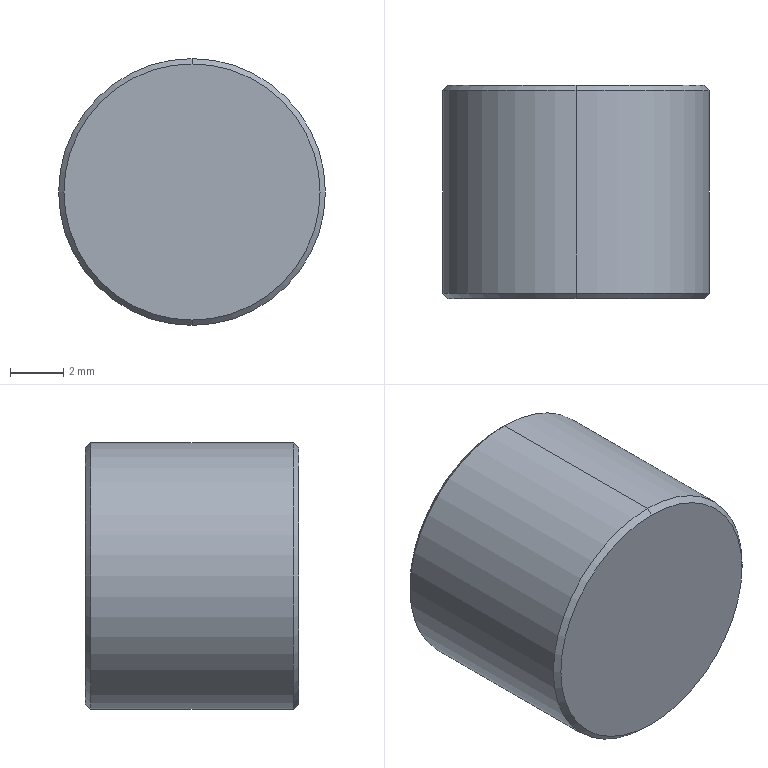Part | SolidWorks | features Chamfer 1, Extrusion 1 | 1 solid | 8 faces | box 10 x 8 x 10 mm | volume 627.079 mm3 | cone 4 | cylinder 2 | plane 2 | commonest cylinder face diameters 10 x2
STEP:
#1=CARTESIAN_POINT('',(0.,8.,4.8));
#2=VERTEX_POINT('',#1);
#3=CARTESIAN_POINT('',(0.,8.,-4.8));
#4=VERTEX_POINT('',#3);
#5=CARTESIAN_POINT('',(0.,8.,0.));
#6=DIRECTION('',(0.,1.,0.));
#7=DIRECTION('',(0.,0.,1.));
#8=AXIS2_PLACEMENT_3D('',#5,#6,#7);
#9=CIRCLE('',#8,4.8);
#10=EDGE_CURVE('',#2,#4,#9,.T.);
#11=ORIENTED_EDGE('',*,*,#10,.F.);
#12=CARTESIAN_POINT('',(0.,7.8,5.));
#13=VERTEX_POINT('',#12);
#14=CARTESIAN_POINT('',(0.,8.,4.8));
#15=DIRECTION('',(0.,-0.7071,0.7071));
#16=VECTOR('',#15,1000.);
#17=LINE('',#14,#16);
#18=EDGE_CURVE('',#2,#13,#17,.T.);
#19=ORIENTED_EDGE('',*,*,#18,.T.);
#20=CARTESIAN_POINT('',(0.,7.8,-5.));
#21=VERTEX_POINT('',#20);
#22=CARTESIAN_POINT('',(0.,7.8,0.));
#23=DIRECTION('',(0.,-1.,0.));
#24=DIRECTION('',(0.,0.,1.));
#25=AXIS2_PLACEMENT_3D('',#22,#23,#24);
#26=CIRCLE('',#25,5.);
#27=EDGE_CURVE('',#21,#13,#26,.T.);
#28=ORIENTED_EDGE('',*,*,#27,.F.);
#29=CARTESIAN_POINT('',(0.,8.,-4.8));
#30=DIRECTION('',(0.,-0.7071,-0.7071));
#31=VECTOR('',#30,1000.);
#32=LINE('',#29,#31);
#33=EDGE_CURVE('',#4,#21,#32,.T.);
#34=ORIENTED_EDGE('',*,*,#33,.F.);
#35=EDGE_LOOP('',(#11,#19,#28,#34));
#36=FACE_OUTER_BOUND('',#35,.T.);
#37=CARTESIAN_POINT('',(0.,8.,0.));
#38=DIRECTION('',(0.,-1.,0.));
#39=DIRECTION('',(0.,0.,-1.));
#40=AXIS2_PLACEMENT_3D('',#37,#38,#39);
#41=CONICAL_SURFACE('',#40,4.8,0.7854);
#42=ADVANCED_FACE('',(#36),#41,.T.);
#43=CARTESIAN_POINT('',(0.,0.,-4.8));
#44=VERTEX_POINT('',#43);
#45=CARTESIAN_POINT('',(0.,0.,4.8));
#46=VERTEX_POINT('',#45);
#47=CARTESIAN_POINT('',(0.,0.,0.));
#48=DIRECTION('',(0.,-1.,0.));
#49=DIRECTION('',(0.,0.,1.));
#50=AXIS2_PLACEMENT_3D('',#47,#48,#49);
#51=CIRCLE('',#50,4.8);
#52=EDGE_CURVE('',#44,#46,#51,.T.);
#53=ORIENTED_EDGE('',*,*,#52,.F.);
#54=CARTESIAN_POINT('',(0.,0.2,-5.));
#55=VERTEX_POINT('',#54);
#56=CARTESIAN_POINT('',(0.,0.2,-5.));
#57=DIRECTION('',(0.,0.7071,-0.7071));
#58=VECTOR('',#57,1000.);
#59=LINE('',#56,#58);
#60=EDGE_CURVE('',#44,#55,#59,.T.);
#61=ORIENTED_EDGE('',*,*,#60,.T.);
#62=CARTESIAN_POINT('',(0.,0.2,5.));
#63=VERTEX_POINT('',#62);
#64=CARTESIAN_POINT('',(0.,0.2,0.));
#65=DIRECTION('',(0.,1.,0.));
#66=DIRECTION('',(0.,0.,1.));
#67=AXIS2_PLACEMENT_3D('',#64,#65,#66);
#68=CIRCLE('',#67,5.);
#69=EDGE_CURVE('',#63,#55,#68,.T.);
#70=ORIENTED_EDGE('',*,*,#69,.F.);
#71=CARTESIAN_POINT('',(0.,0.2,5.));
#72=DIRECTION('',(0.,0.7071,0.7071));
#73=VECTOR('',#72,1000.);
#74=LINE('',#71,#73);
#75=EDGE_CURVE('',#46,#63,#74,.T.);
#76=ORIENTED_EDGE('',*,*,#75,.F.);
#77=EDGE_LOOP('',(#53,#61,#70,#76));
#78=FACE_OUTER_BOUND('',#77,.T.);
#79=CARTESIAN_POINT('',(0.,0.2,0.));
#80=DIRECTION('',(0.,1.,0.));
#81=DIRECTION('',(0.,0.,1.));
#82=AXIS2_PLACEMENT_3D('',#79,#80,#81);
#83=CONICAL_SURFACE('',#82,5.,0.7854);
#84=ADVANCED_FACE('',(#78),#83,.T.);
#85=ORIENTED_EDGE('',*,*,#27,.T.);
#86=CARTESIAN_POINT('',(0.,8.,5.));
#87=DIRECTION('',(0.,-1.,0.));
#88=VECTOR('',#87,1000.);
#89=LINE('',#86,#88);
#90=EDGE_CURVE('',#13,#63,#89,.T.);
#91=ORIENTED_EDGE('',*,*,#90,.T.);
#92=ORIENTED_EDGE('',*,*,#69,.T.);
#93=CARTESIAN_POINT('',(0.,8.,-5.));
#94=DIRECTION('',(0.,-1.,0.));
#95=VECTOR('',#94,1000.);
#96=LINE('',#93,#95);
#97=EDGE_CURVE('',#21,#55,#96,.T.);
#98=ORIENTED_EDGE('',*,*,#97,.F.);
#99=EDGE_LOOP('',(#85,#91,#92,#98));
#100=FACE_OUTER_BOUND('',#99,.T.);
#101=CARTESIAN_POINT('',(0.,8.,0.));
#102=DIRECTION('',(0.,-1.,0.));
#103=DIRECTION('',(0.,0.,-1.));
#104=AXIS2_PLACEMENT_3D('',#101,#102,#103);
#105=CYLINDRICAL_SURFACE('',#104,5.);
#106=ADVANCED_FACE('',(#100),#105,.T.);
#107=ORIENTED_EDGE('',*,*,#90,.F.);
#108=CARTESIAN_POINT('',(0.,7.8,0.));
#109=DIRECTION('',(0.,-1.,0.));
#110=DIRECTION('',(0.,0.,1.));
#111=AXIS2_PLACEMENT_3D('',#108,#109,#110);
#112=CIRCLE('',#111,5.);
#113=EDGE_CURVE('',#13,#21,#112,.T.);
#114=ORIENTED_EDGE('',*,*,#113,.T.);
#115=ORIENTED_EDGE('',*,*,#97,.T.);
#116=CARTESIAN_POINT('',(0.,0.2,0.));
#117=DIRECTION('',(0.,1.,0.));
#118=DIRECTION('',(0.,0.,1.));
#119=AXIS2_PLACEMENT_3D('',#116,#117,#118);
#120=CIRCLE('',#119,5.);
#121=EDGE_CURVE('',#55,#63,#120,.T.);
#122=ORIENTED_EDGE('',*,*,#121,.T.);
#123=EDGE_LOOP('',(#107,#114,#115,#122));
#124=FACE_OUTER_BOUND('',#123,.T.);
#125=CARTESIAN_POINT('',(0.,8.,0.));
#126=DIRECTION('',(0.,-1.,0.));
#127=DIRECTION('',(0.,0.,-1.));
#128=AXIS2_PLACEMENT_3D('',#125,#126,#127);
#129=CYLINDRICAL_SURFACE('',#128,5.);
#130=ADVANCED_FACE('',(#124),#129,.T.);
#131=CARTESIAN_POINT('',(0.,8.,0.));
#132=DIRECTION('',(0.,1.,0.));
#133=DIRECTION('',(0.,0.,1.));
#134=AXIS2_PLACEMENT_3D('',#131,#132,#133);
#135=CIRCLE('',#134,4.8);
#136=EDGE_CURVE('',#4,#2,#135,.T.);
#137=ORIENTED_EDGE('',*,*,#136,.T.);
#138=ORIENTED_EDGE('',*,*,#10,.T.);
#139=EDGE_LOOP('',(#137,#138));
#140=FACE_OUTER_BOUND('',#139,.T.);
#141=CARTESIAN_POINT('',(0.,8.,0.));
#142=DIRECTION('',(0.,1.,0.));
#143=DIRECTION('',(0.,0.,1.));
#144=AXIS2_PLACEMENT_3D('',#141,#142,#143);
#145=PLANE('',#144);
#146=ADVANCED_FACE('',(#140),#145,.T.);
#147=CARTESIAN_POINT('',(0.,0.,0.));
#148=DIRECTION('',(0.,-1.,0.));
#149=DIRECTION('',(0.,0.,1.));
#150=AXIS2_PLACEMENT_3D('',#147,#148,#149);
#151=CIRCLE('',#150,4.8);
#152=EDGE_CURVE('',#46,#44,#151,.T.);
#153=ORIENTED_EDGE('',*,*,#152,.T.);
#154=ORIENTED_EDGE('',*,*,#52,.T.);
#155=EDGE_LOOP('',(#153,#154));
#156=FACE_OUTER_BOUND('',#155,.T.);
#157=CARTESIAN_POINT('',(0.,0.,0.));
#158=DIRECTION('',(0.,1.,0.));
#159=DIRECTION('',(0.,0.,1.));
#160=AXIS2_PLACEMENT_3D('',#157,#158,#159);
#161=PLANE('',#160);
#162=ADVANCED_FACE('',(#156),#161,.F.);
#163=ORIENTED_EDGE('',*,*,#60,.F.);
#164=ORIENTED_EDGE('',*,*,#152,.F.);
#165=ORIENTED_EDGE('',*,*,#75,.T.);
#166=ORIENTED_EDGE('',*,*,#121,.F.);
#167=EDGE_LOOP('',(#163,#164,#165,#166));
#168=FACE_OUTER_BOUND('',#167,.T.);
#169=CARTESIAN_POINT('',(0.,0.2,0.));
#170=DIRECTION('',(0.,1.,0.));
#171=DIRECTION('',(0.,0.,1.));
#172=AXIS2_PLACEMENT_3D('',#169,#170,#171);
#173=CONICAL_SURFACE('',#172,5.,0.7854);
#174=ADVANCED_FACE('',(#168),#173,.T.);
#175=ORIENTED_EDGE('',*,*,#18,.F.);
#176=ORIENTED_EDGE('',*,*,#136,.F.);
#177=ORIENTED_EDGE('',*,*,#33,.T.);
#178=ORIENTED_EDGE('',*,*,#113,.F.);
#179=EDGE_LOOP('',(#175,#176,#177,#178));
#180=FACE_OUTER_BOUND('',#179,.T.);
#181=CARTESIAN_POINT('',(0.,8.,0.));
#182=DIRECTION('',(0.,-1.,0.));
#183=DIRECTION('',(0.,0.,-1.));
#184=AXIS2_PLACEMENT_3D('',#181,#182,#183);
#185=CONICAL_SURFACE('',#184,4.8,0.7854);
#186=ADVANCED_FACE('',(#180),#185,.T.);
#187=CLOSED_SHELL('',(#42,#84,#106,#130,#146,#162,#174,#186));
#188=MANIFOLD_SOLID_BREP('',#187);
#189=CARTESIAN_POINT('',(0.,0.,0.));
#190=DIRECTION('',(0.,0.,1.));
#191=DIRECTION('',(1.,0.,0.));
#192=AXIS2_PLACEMENT_3D('',#189,#190,#191);
#193=(LENGTH_UNIT()NAMED_UNIT(*)SI_UNIT(.MILLI.,.METRE.));
#194=UNCERTAINTY_MEASURE_WITH_UNIT(LENGTH_MEASURE(0.00001),#193,'','');
#195=(NAMED_UNIT(*)PLANE_ANGLE_UNIT()SI_UNIT($,.RADIAN.));
#196=(NAMED_UNIT(*)SI_UNIT($,.STERADIAN.)SOLID_ANGLE_UNIT());
#197=(GEOMETRIC_REPRESENTATION_CONTEXT(3)GLOBAL_UNCERTAINTY_ASSIGNED_CONTEXT((#194))GLOBAL_UNIT_ASSIGNED_CONTEXT((#193,#195,#196))REPRESENTATION_CONTEXT('',''));
#198=ADVANCED_BREP_SHAPE_REPRESENTATION('',(#188,#192),#197);